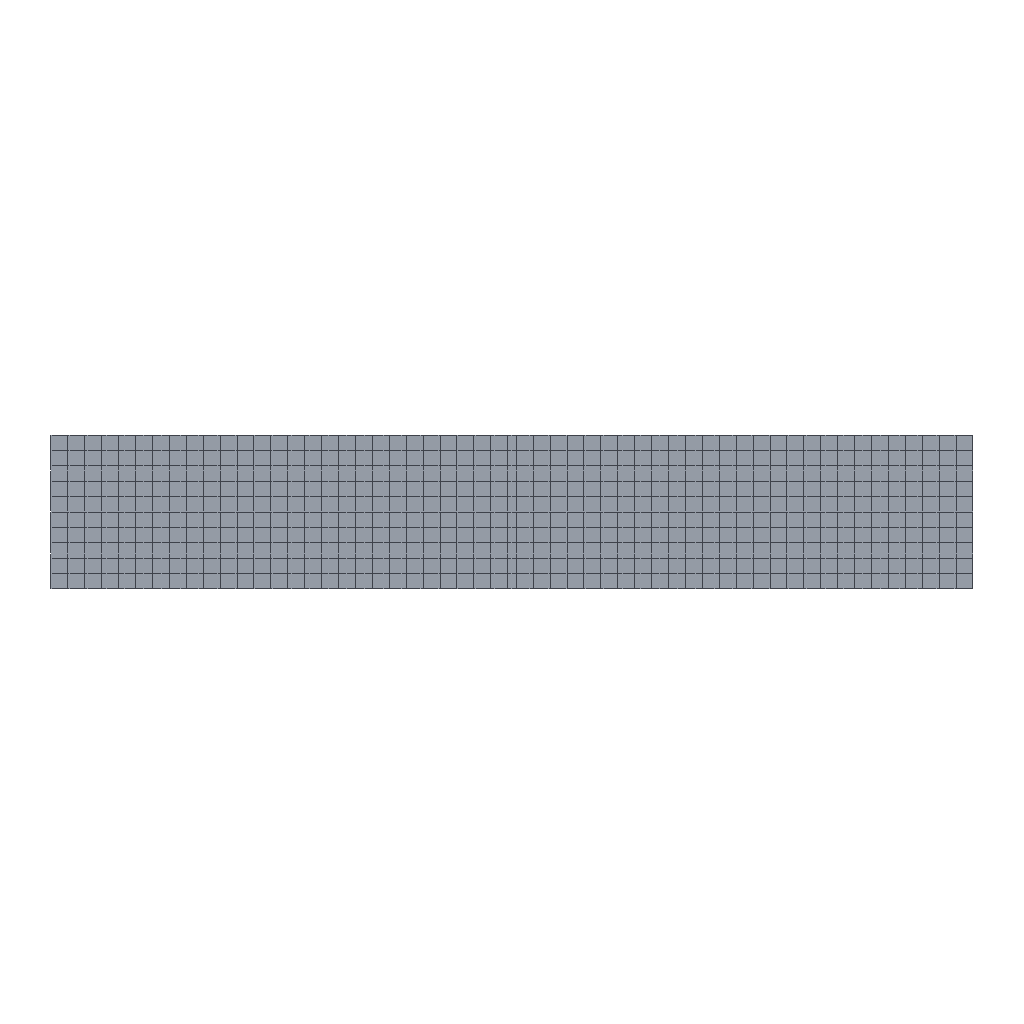Simulation study | abaqus
Set-up summary:
category,name,step,type,value,unit,region
solver,abaqus,,Abaqus/CAE 2024
units,unstated,,unstated,E=10000 density=0.8 (no match)
analysis,Step-1,,soils,time_period=1
mesh,nodes,,,616
mesh,elements,,,550
element_type,CPE4P,,,545
element_type,CPE4,,,5
material,soil,,E,10000
material,soil,,nu,0.3
material,soil,,density,0.8
material,wall,,E,2e+07
material,wall,,nu,0.2
material,wall,,density,2.4
section,soil,,solid section,,,soil
section,wall,,solid section,,,wall
load,Predefined,initial,initial condition ratio
load,Load-1,Step-1,gravity,10,,whole model
bc,BC-1,Step-1,fixed,"[dofs=x,y n=2]",,_PickedSet4
bc,BC-2,Step-1,displacement,30 [dofs=8],,_PickedSet5_PP_
bc,BC-3,Step-1,fixed,[dofs=8],,_PickedSet6_PP_
Abaqus input file, long lists of numbers shortened:
*Heading
** Job name: deck Model name: Model-1
** Generated by: Abaqus/CAE 2024
*Preprint, echo=NO, model=NO, history=NO, contact=NO
**
** PARTS
**
*Part, name=Part-1
*Node
      1,        27.25,          4.5
      2,          54.,          4.5
** (614 more lines like these left out)
*Element, type=CPE4P
  1,   1,  13, 201,  72
  2,  13,  14, 202, 201
** (543 more lines like these left out)
*Element, type=CPE4
411,  10, 140,  69,   4
412, 140, 139,  70,  69
** (3 more lines like these left out)
*Nset, nset=soil, generate
   1,  616,    1
*Elset, elset=soil
   1,   2,   3,   4,   5,   6,   7,   8,   9,  10,  11,  12,  13,  14,  15,  16
  17,  18,  19,  20,  21,  22,  23,  24,  25,  26,  27,  28,  29,  30,  31,  32
** (33 more lines like these left out)
*Nset, nset=wall
   1,   4,   7,  10,  69,  70,  71,  72, 137, 138, 139, 140
*Elset, elset=wall, generate
 411,  415,    1
** Section: soil
*Solid Section, elset=soil, material=soil
,
** Section: wall
*Solid Section, elset=wall, material=wall
,
*End Part
**
**
** ASSEMBLY
**
*Assembly, name=Assembly
**
*Instance, name=Part-1-1, part=Part-1
*End Instance
**
*Nset, nset=_PickedSet4, internal, instance=Part-1-1, generate
   1,  616,    1
*Elset, elset=_PickedSet4, internal, instance=Part-1-1, generate
   1,  550,    1
*Nset, nset=_PickedSet5, internal, instance=Part-1-1
  10,  11, 141, 142, 143, 144, 145, 146, 147, 148, 149, 150, 151, 152, 153, 154
 155, 156, 157, 158, 159, 160, 161, 162, 163, 164, 165, 166
*Elset, elset=_PickedSet5, internal, instance=Part-1-1, generate
 384,  410,    1
*Nset, nset=_PickedSet6, internal, instance=Part-1-1
  3,  4, 43, 44, 45, 46, 47, 48, 49, 50, 51, 52, 53, 54, 55, 56
 57, 58, 59, 60, 61, 62, 63, 64, 65, 66, 67, 68
*Elset, elset=_PickedSet6, internal, instance=Part-1-1, generate
 109,  135,    1
*Nset, nset=_PickedSet5_PP_, internal, instance=Part-1-1
  10,  11, 141, 142, 143, 144, 145, 146, 147, 148, 149, 150, 151, 152, 153, 154
 155, 156, 157, 158, 159, 160, 161, 162, 163, 164, 165, 166
*Nset, nset=_PickedSet6_PP_, internal, instance=Part-1-1
  3,  4, 43, 44, 45, 46, 47, 48, 49, 50, 51, 52, 53, 54, 55, 56
 57, 58, 59, 60, 61, 62, 63, 64, 65, 66, 67, 68
*End Assembly
**
** MATERIALS
**
*Material, name=soil
*Density
 0.8,
*Elastic
10000., 0.3
*Permeability, specific=10.
 5e-05,0.
*Material, name=wall
*Density
 2.4,
*Elastic
 2e+07, 0.2
**
** PREDEFINED FIELDS
**
** Name: Predefined Field-1   Type: Void ratio
*Initial Conditions, TYPE=RATIO
Part-1-1.soil, 1.
** ----------------------------------------------------------------
**
** STEP: Step-1
**
*Step, name=Step-1, nlgeom=NO
*Soils, utol=1.0, creep=none
1., 1., 1e-05, 1.,
**
** BOUNDARY CONDITIONS
**
** Name: BC-1 Type: Displacement/Rotation
*Boundary
_PickedSet4, 1, 1
_PickedSet4, 2, 2
** Name: BC-2 Type: Pore pressure
*Boundary
_PickedSet5_PP_, 8, 8, 30.
** Name: BC-3 Type: Pore pressure
*Boundary
_PickedSet6_PP_, 8, 8
**
** LOADS
**
** Name: Load-1   Type: Gravity
*Dload
, GRAV, 10., 0., -1.
**
** OUTPUT REQUESTS
**
*Restart, write, frequency=0
**
** FIELD OUTPUT: F-Output-1
**
*Output, field
*Node Output
CF, COORD, POR, RF, RVF, U
*Element Output, directions=YES
COORD, FLVEL, LE, S, SAT, VOIDR
*Contact Output
PFL, PFLA, PTL, PTLA
**
** HISTORY OUTPUT: H-Output-1
**
*Output, history, variable=PRESELECT
*End Step
Results summary:
result,odb.job_status,,,JOB_STATUS_COMPLETED_SUCCESSFULLY,"consistent, unstated (Abaqus has no unit system)"
result,steps[0].procedure,Step-1,,*SOILS,"consistent, unstated (Abaqus has no unit system)"
result,steps[0].time_period,Step-1,,1,"consistent, unstated (Abaqus has no unit system)"
result,steps[0].n_frames,Step-1,,2,"consistent, unstated (Abaqus has no unit system)"
result,steps[0].last_frame.id,Step-1,,1,"consistent, unstated (Abaqus has no unit system)"
result,steps[0].last_frame.value,Step-1,,1,"consistent, unstated (Abaqus has no unit system)"
result,steps[0].last_frame.description,Step-1,,Increment      1: Step Time =    1.000,"consistent, unstated (Abaqus has no unit system)"
result,steps[0].completed,Step-1,,True,"consistent, unstated (Abaqus has no unit system)"
result,steps[0].max_U_magnitude,Step-1,,0,"consistent, unstated (Abaqus has no unit system)"
result,steps[0].max_S_mises,Step-1,,2.91093e-27,"consistent, unstated (Abaqus has no unit system)"
result,steps[0].RF_sum[1],Step-1,,8.57105e-05,"consistent, unstated (Abaqus has no unit system)"
result,steps[0].RF_sum[2],Step-1,,6342.75,"consistent, unstated (Abaqus has no unit system)"